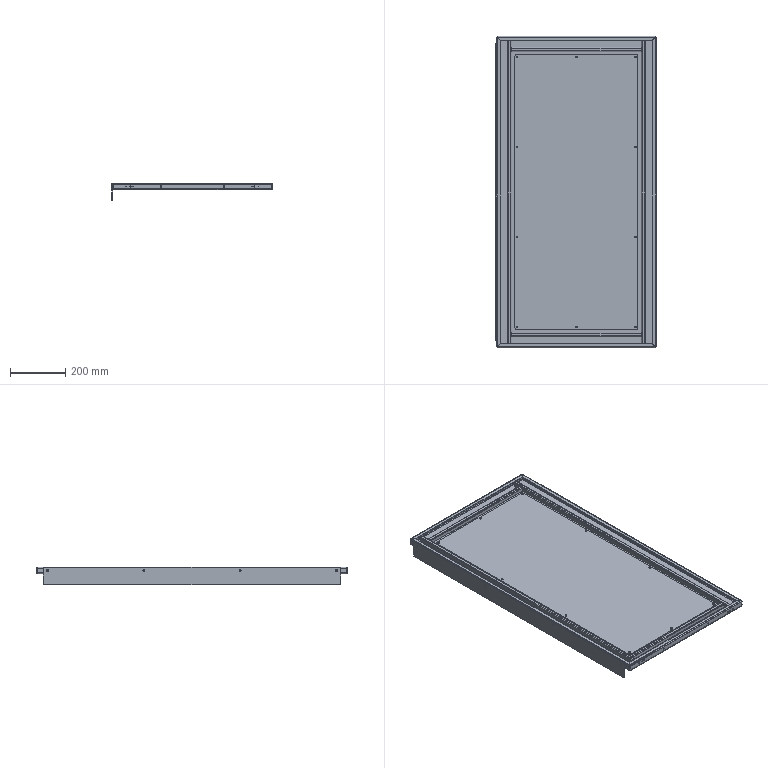Part | NX | features BREP 7 | 7 solids | 304 faces | box 583 x 1130 x 65 mm | volume 3365966 mm3 | plane 136 | cylinder 132 | cone 20 | spline 16 | commonest cylinder face diameters 4.2 x24 4 x20 5 x20 5.8 x20 3.3 x16 6 x8